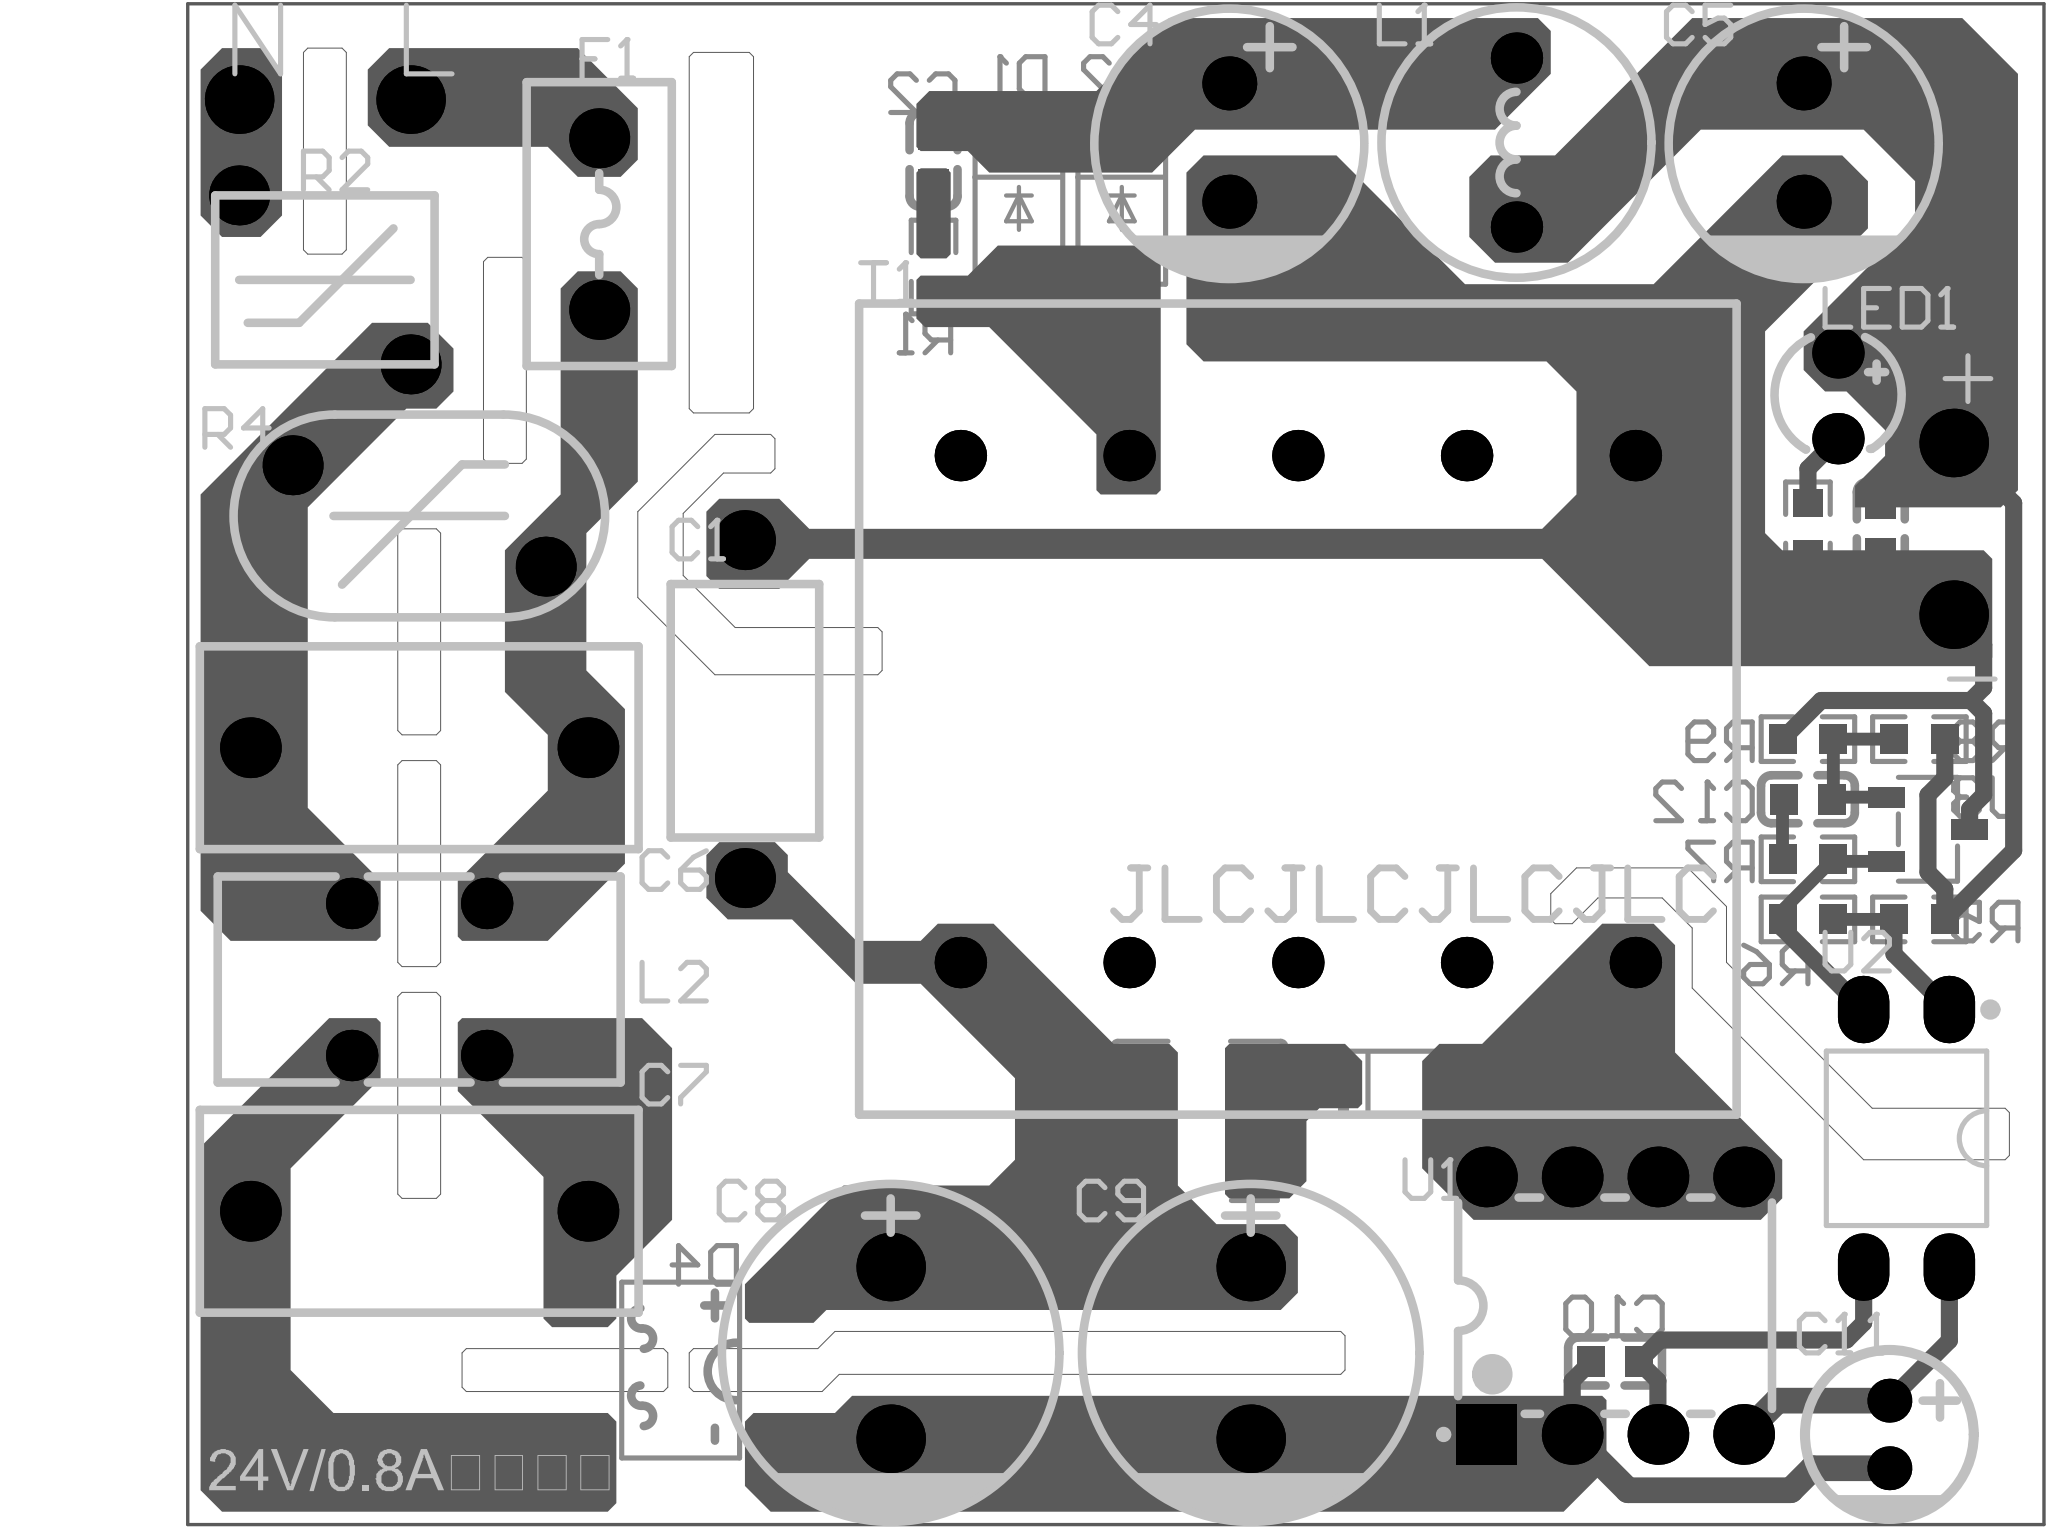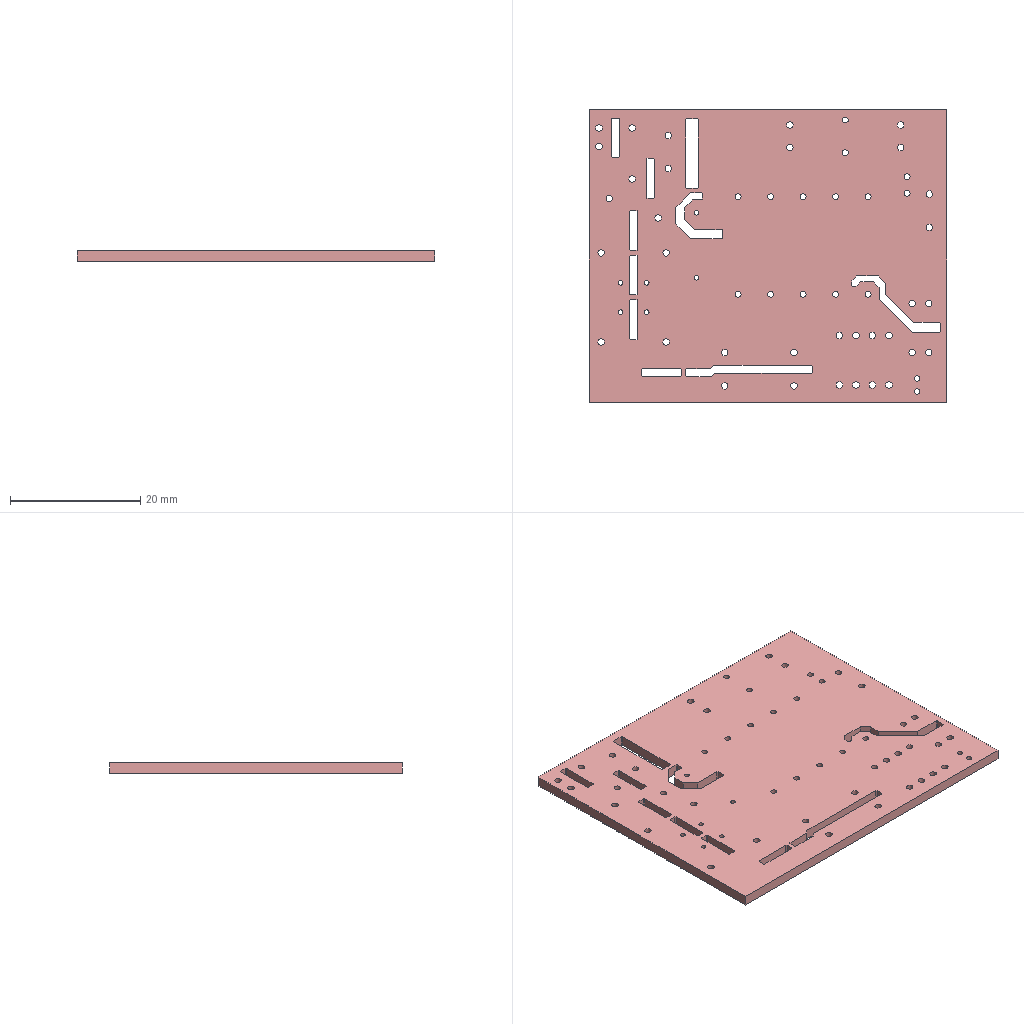Circuit board layout | Altium Designer | box 55 x 45 x 1.6 mm
Layer stack:
# Altium Designer layer stack of  (unit mm; dielectric type: 0 none, 1 core, 2 prepreg, 3 surface material)
index,name,kind,layer,copper_thickness_mm,dielectric_type,dielectric_thickness_mm,dielectric_material,dielectric_constant
0,Top Paste Mask Layer,other,,,,,,
1,Top Silkscreen Layer,other,,,,,,
2,Top Solder Mask Layer,dielectric,,,3,0.01,,3.3
3,Top Layer,copper,Top Layer,0.035,,,,
4,Dielectric1,dielectric,,,3,1.51,FR4,4.5
5,Bottom Layer,copper,Bottom Layer,0.035,,,,
6,Bottom Solder Mask Layer,dielectric,,,3,0.01,,3.3
7,Bottom Silkscreen Layer,other,,,,,,
8,Bottom Paste Mask Layer,other,,,,,,
# drill layer pairs: low layer,high layer
drill_pair,Top Layer,Bottom Layer
Part placement:
Designator,Comment,Layer,Footprint,Center-X(mm),Center-Y(mm),Rotation
C1,1nF,TopLayer,CAP-TH_L7.5-W4.5-P10.00-D0.6,92.71,100.33,90
C2,100nF,BottomLayer,C0603,98.298,116.586,90
C3,10nF,BottomLayer,C1206,106.172,89.408,180
C4,470uF,TopLayer,CAP-TH_BD8.0-P3.50-D0.6-FD,107.061,117.094,270
C5,470uF,TopLayer,CAP-TH_BD8.0-P3.50-D0.6-FD,124.079,117.094,270
C6,100nF,TopLayer,CAP-TH_L13.0-W6.0-P10.00-D0.6,83.058,99.187,0
C7,100nF,TopLayer,CAP-TH_L13.0-W6.0-P10.00-D0.6,83.058,85.471,0
C8,22uF,TopLayer,CAP-TH_BD10.0-P5.00-D1.0-FD,97.028,81.28,270
C9,22uF,TopLayer,CAP-TH_BD10.0-P5.00-D1.0-FD,107.696,81.28,270
C10,1nF,BottomLayer,C0603,118.491,81.026,0
C11,47uF,TopLayer,CAP-TH_BD5.0-P2.00-D0.8-FD,126.619,78.867,270
C12,100nF,BottomLayer,C0603,124.206,97.663,180
D1,SS310,BottomLayer,SMA_L4.3-W2.6-LS5.0-FD,100.838,115.062,90
D2,SS310,BottomLayer,SMA_L4.3-W2.6-LS5.0-FD,103.886,115.062,90
D3,FR107W,BottomLayer,SOD-123FL_L2.7-W1.8-LS3.8-RD,111.887,89.281,0
D4,ABS210,BottomLayer,ABF_L5.1-W4.4-P4.00-LS6.2-BL,90.805,80.772,90
F1,MST 2.5A 250V,TopLayer,FUSE-TH_L8.4-W4.3-P5.08-D1.0,88.392,114.681,270
L1,10uH,TopLayer,IND-TH_BD8.0-P5.00-D0.7,115.57,117.094,270
L2,PDMCAT953-102MLN,TopLayer,IND-TH_4P-L12.0-W6.0_PDMCAT953-501MLN,83.058,92.329,180
C13,100nF,BottomLayer,C0603,126.365,105.664,90
R1,10K,BottomLayer,R0603,98.298,113.411,90
R2,NTC33D-7,TopLayer,RES-TH_L6.5-W5.0-P5.00-D0.6-S4.40,80.264,113.03,0
R3,100K,BottomLayer,R1206,106.172,86.868,180
R4,10D471K,TopLayer,RES-TH_L11.0-W6.0-P7.50-D0.8-S3.00,83.058,106.045,180
R5,1.5K,BottomLayer,R0603,127.508,94.107,0
R6,1.5K,BottomLayer,R0603,124.206,94.107,0
R7,10K,BottomLayer,R0603,124.206,95.885,180
R8,20K,BottomLayer,R0603,127.508,99.441,0
R9,2.2K,BottomLayer,R0603,124.206,99.441,0
T1,,TopLayer,EE25_5+5,109.093,100.33,90
U1,DK125,TopLayer,DIP-8_L9.2-W6.4-P2.54-LS7.6-BL,118.491,82.677,0
U2,PC817C,TopLayer,DIP-4_L4.6-W6.5-P2.54-LS7.6-BL,127.127,87.63,180
U3,TL431AIDBZR,BottomLayer,SOT-23-3_L2.9-W1.6-P1.90-LS2.8-BR,127.762,96.774,180
LED1,XL-302UGD,TopLayer,LED-TH_BD3.8-P2.54-FD_GREEN,125.095,109.601,270
R10,4.7K,BottomLayer,R0603,124.206,105.664,90
Pad and via stacks:
# Altium Designer via and pad stacks of  (unit mm). Each distinct definition once, with the count of objects using it.
# via: kind,start_layer,end_layer,hole_mm,diameter_mm,mode(0 simple;1 top-mid-bottom;2 full stack),diameter_per_layer,count,example_net
# pad: kind,layer,hole_mm,hole_type(0 round;1 square;2 slot),plating,top_size,top_shape(1 round;2 rect;3 octagon;9 rounded rect),mid_size,bottom_size,mode,footprint,size_per_layer,count,example
pad,Multi-Layer,1.001,0,plated,2.032x2.032,1,2.032x2.032,2.032x2.032,0,,,4,1
pad,Multi-Layer,0.7,0,plated,1.778x1.778,1,1.778x1.778,1.778x1.778,0,CAP-TH_L7.5-W4.5-P10.00-D0.6,,2,C1.1
pad,Multi-Layer,1,0,plated,1.6x1.6,1,1.6x1.6,1.6x1.6,0,CAP-TH_BD8.0-P3.50-D0.6-FD,,4,C4.2
pad,Multi-Layer,1,0,plated,1.8x1.8,1,1.8x1.8,1.8x1.8,0,CAP-TH_L13.0-W6.0-P10.00-D0.6,,4,C6.1
pad,Multi-Layer,1,0,plated,2.032x2.032,1,2.032x2.032,2.032x2.032,0,CAP-TH_BD10.0-P5.00-D1.0-FD,,4,C8.1
pad,Multi-Layer,0.8,0,plated,1.3x1.3,1,1.3x1.3,1.3x1.3,0,CAP-TH_BD5.0-P2.00-D0.8-FD,,2,C11.1
pad,Multi-Layer,1,0,plated,1.778x1.778,1,1.778x1.778,1.778x1.778,0,FUSE-TH_L8.4-W4.3-P5.08-D1.0,,2,F1.1
pad,Multi-Layer,0.91,0,plated,1.52x1.52,1,1.52x1.52,1.52x1.52,0,IND-TH_BD8.0-P5.00-D0.7,,2,L1.2
pad,Multi-Layer,0.7,0,plated,1.524x1.524,1,1.524x1.524,1.524x1.524,0,IND-TH_4P-L12.0-W6.0_PDMCAT953-501MLN,,4,L2.1
pad,Multi-Layer,1,0,plated,1.778x1.778,1,1.778x1.778,1.778x1.778,0,RES-TH_L6.5-W5.0-P5.00-D0.6-S4.40,,2,R2.1
pad,Multi-Layer,1,0,plated,1.778x1.778,1,1.778x1.778,1.778x1.778,0,RES-TH_L11.0-W6.0-P7.50-D0.8-S3.00,,2,R4.1
pad,Multi-Layer,0.9144,0,plated,1.524x1.524,1,1.524x1.524,1.524x1.524,0,EE25 5+5,,10,T1.1
pad,Multi-Layer,1,0,plated,1.8x1.8,1,1.8x1.8,1.8x1.8,0,DIP-8_L9.2-W6.4-P2.54-LS7.6-BL,,7,U1.8
pad,Multi-Layer,1,0,plated,1.8x1.8,2,1.8x1.8,1.8x1.8,0,DIP-8_L9.2-W6.4-P2.54-LS7.6-BL,,1,U1.1
pad,Multi-Layer,1,0,plated,1.524x2,1,1.524x2,1.524x2,0,DIP-4_L4.6-W6.5-P2.54-LS7.6-BL,,4,U2.1
pad,Multi-Layer,0.9,0,plated,1.524x1.524,1,1.524x1.524,1.524x1.524,0,LED-TH_BD3.8-P2.54-FD_GREEN,,2,LED1.1
pad,Bottom Layer,0,0,plated,0.8x0.9,2,0.8x0.9,0.8x0.9,0,C0603,,8,C2.2
pad,Bottom Layer,0,0,plated,1.485x1.728,2,1.485x1.728,1.485x1.728,0,C1206,,2,C3.2
pad,Bottom Layer,0,0,plated,2.046x1.62,2,2.046x1.62,2.046x1.62,0,SMA_L4.3-W2.6-LS5.0-FD,,4,D1.1
pad,Bottom Layer,0,0,plated,1.4x1.2,2,1.4x1.2,1.4x1.2,0,SOD-123FL_L2.7-W1.8-LS3.8-RD,,2,D3.2
pad,Bottom Layer,0,0,plated,0.84x1.695,2,0.84x1.695,0.84x1.695,0,ABF_L5.1-W4.4-P4.00-LS6.2-BL,,4,D4.1
pad,Bottom Layer,0,0,plated,0.8065x0.864,2,0.8065x0.864,0.8065x0.864,0,R0603,,14,R1.2
pad,Bottom Layer,0,0,plated,1.208x1.701,2,1.208x1.701,1.208x1.701,0,R1206,,2,R3.2
pad,Bottom Layer,0,0,plated,1.07x0.6,2,1.07x0.6,1.07x0.6,0,SOT-23-3_L2.9-W1.6-P1.90-LS2.8-BR,,3,U3.1